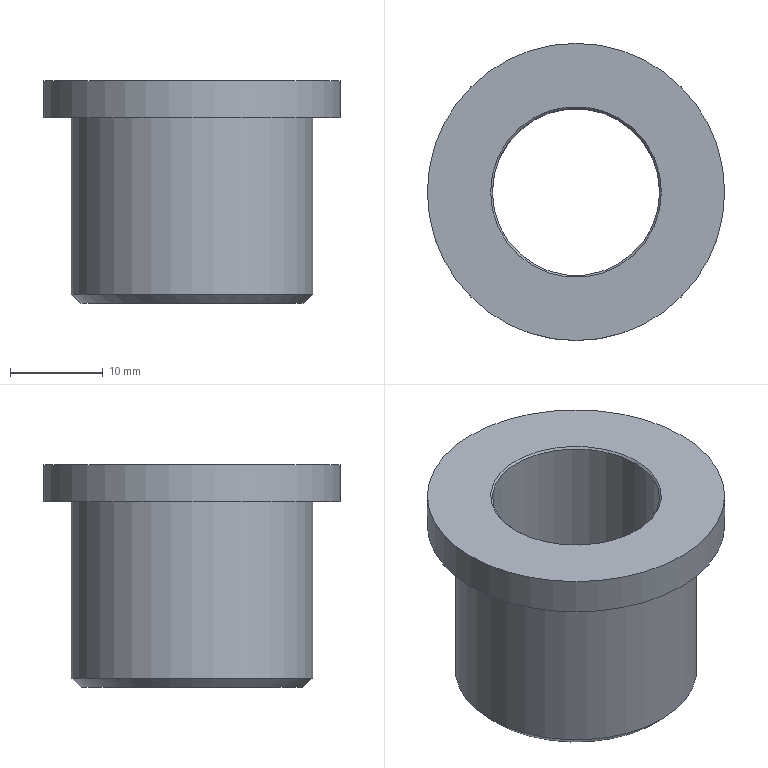Part | NX | features CHAMFER 2, DATUM_CSYS 2, EXTRUDE 2, SKETCH 1 | 1 solid | 9 faces | box 32 x 32 x 24 mm | volume 7686 mm3 | cylinder 3 | plane 3 | cone 3 | commonest cylinder face diameters 18 x1 26 x1 32 x1
STEP:
#1=CARTESIAN_POINT('',(16.,0.,4.));
#2=VERTEX_POINT('',#1);
#3=CARTESIAN_POINT('',(0.,0.,4.));
#4=DIRECTION('',(0.,0.,1.));
#5=DIRECTION('',(1.,0.,0.));
#6=AXIS2_PLACEMENT_3D('',#3,#4,#5);
#7=CIRCLE('',#6,16.);
#8=EDGE_CURVE('',#2,#2,#7,.T.);
#9=ORIENTED_EDGE('',*,*,#8,.F.);
#10=EDGE_LOOP('',(#9));
#11=FACE_BOUND('',#10,.T.);
#12=CARTESIAN_POINT('',(16.,0.,0.));
#13=VERTEX_POINT('',#12);
#14=CARTESIAN_POINT('',(0.,0.,0.));
#15=DIRECTION('',(0.,0.,1.));
#16=DIRECTION('',(1.,0.,0.));
#17=AXIS2_PLACEMENT_3D('',#14,#15,#16);
#18=CIRCLE('',#17,16.);
#19=EDGE_CURVE('',#13,#13,#18,.T.);
#20=ORIENTED_EDGE('',*,*,#19,.T.);
#21=EDGE_LOOP('',(#20));
#22=FACE_BOUND('',#21,.T.);
#23=CARTESIAN_POINT('',(0.,0.,4.));
#24=DIRECTION('',(0.,0.,-1.));
#25=DIRECTION('',(-1.,0.,0.));
#26=AXIS2_PLACEMENT_3D('',#23,#24,#25);
#27=CYLINDRICAL_SURFACE('',#26,16.);
#28=ADVANCED_FACE('',(#11,#22),#27,.T.);
#29=CARTESIAN_POINT('',(-9.,0.,-19.8));
#30=VERTEX_POINT('',#29);
#31=CARTESIAN_POINT('',(0.,0.,-19.8));
#32=DIRECTION('',(0.,0.,-1.));
#33=DIRECTION('',(-1.,0.,0.));
#34=AXIS2_PLACEMENT_3D('',#31,#32,#33);
#35=CIRCLE('',#34,9.);
#36=EDGE_CURVE('',#30,#30,#35,.T.);
#37=ORIENTED_EDGE('',*,*,#36,.T.);
#38=EDGE_LOOP('',(#37));
#39=FACE_BOUND('',#38,.T.);
#40=CARTESIAN_POINT('',(9.,0.,3.8));
#41=VERTEX_POINT('',#40);
#42=CARTESIAN_POINT('',(0.,0.,3.8));
#43=DIRECTION('',(0.,0.,1.));
#44=DIRECTION('',(1.,0.,0.));
#45=AXIS2_PLACEMENT_3D('',#42,#43,#44);
#46=CIRCLE('',#45,9.);
#47=EDGE_CURVE('',#41,#41,#46,.T.);
#48=ORIENTED_EDGE('',*,*,#47,.T.);
#49=EDGE_LOOP('',(#48));
#50=FACE_BOUND('',#49,.T.);
#51=CARTESIAN_POINT('',(0.,0.,4.));
#52=DIRECTION('',(0.,0.,-1.));
#53=DIRECTION('',(-1.,0.,0.));
#54=AXIS2_PLACEMENT_3D('',#51,#52,#53);
#55=CYLINDRICAL_SURFACE('',#54,9.);
#56=ADVANCED_FACE('',(#39,#50),#55,.F.);
#57=CARTESIAN_POINT('',(9.2,0.,4.));
#58=VERTEX_POINT('',#57);
#59=CARTESIAN_POINT('',(0.,0.,4.));
#60=DIRECTION('',(0.,0.,1.));
#61=DIRECTION('',(1.,0.,0.));
#62=AXIS2_PLACEMENT_3D('',#59,#60,#61);
#63=CIRCLE('',#62,9.2);
#64=EDGE_CURVE('',#58,#58,#63,.F.);
#65=ORIENTED_EDGE('',*,*,#64,.T.);
#66=EDGE_LOOP('',(#65));
#67=FACE_BOUND('',#66,.T.);
#68=ORIENTED_EDGE('',*,*,#8,.T.);
#69=EDGE_LOOP('',(#68));
#70=FACE_BOUND('',#69,.T.);
#71=CARTESIAN_POINT('',(0.,0.,4.));
#72=DIRECTION('',(0.,0.,1.));
#73=DIRECTION('',(1.,0.,0.));
#74=AXIS2_PLACEMENT_3D('',#71,#72,#73);
#75=PLANE('',#74);
#76=ADVANCED_FACE('',(#67,#70),#75,.T.);
#77=CARTESIAN_POINT('',(13.,0.,0.));
#78=VERTEX_POINT('',#77);
#79=CARTESIAN_POINT('',(0.,0.,0.));
#80=DIRECTION('',(0.,0.,-1.));
#81=DIRECTION('',(1.,0.,0.));
#82=AXIS2_PLACEMENT_3D('',#79,#80,#81);
#83=CIRCLE('',#82,13.);
#84=EDGE_CURVE('',#78,#78,#83,.T.);
#85=ORIENTED_EDGE('',*,*,#84,.F.);
#86=EDGE_LOOP('',(#85));
#87=FACE_BOUND('',#86,.T.);
#88=ORIENTED_EDGE('',*,*,#19,.F.);
#89=EDGE_LOOP('',(#88));
#90=FACE_BOUND('',#89,.T.);
#91=CARTESIAN_POINT('',(0.,0.,0.));
#92=DIRECTION('',(0.,0.,1.));
#93=DIRECTION('',(1.,0.,0.));
#94=AXIS2_PLACEMENT_3D('',#91,#92,#93);
#95=PLANE('',#94);
#96=ADVANCED_FACE('',(#87,#90),#95,.F.);
#97=CARTESIAN_POINT('',(-13.,0.,-19.));
#98=VERTEX_POINT('',#97);
#99=CARTESIAN_POINT('',(0.,0.,-19.));
#100=DIRECTION('',(0.,0.,-1.));
#101=DIRECTION('',(-1.,0.,0.));
#102=AXIS2_PLACEMENT_3D('',#99,#100,#101);
#103=CIRCLE('',#102,13.);
#104=EDGE_CURVE('',#98,#98,#103,.F.);
#105=ORIENTED_EDGE('',*,*,#104,.T.);
#106=EDGE_LOOP('',(#105));
#107=FACE_BOUND('',#106,.T.);
#108=ORIENTED_EDGE('',*,*,#84,.T.);
#109=EDGE_LOOP('',(#108));
#110=FACE_BOUND('',#109,.T.);
#111=CARTESIAN_POINT('',(0.,0.,-20.));
#112=DIRECTION('',(0.,0.,1.));
#113=DIRECTION('',(1.,0.,0.));
#114=AXIS2_PLACEMENT_3D('',#111,#112,#113);
#115=CYLINDRICAL_SURFACE('',#114,13.);
#116=ADVANCED_FACE('',(#107,#110),#115,.T.);
#117=CARTESIAN_POINT('',(-9.2,0.,-20.));
#118=VERTEX_POINT('',#117);
#119=CARTESIAN_POINT('',(0.,0.,-20.));
#120=DIRECTION('',(0.,0.,-1.));
#121=DIRECTION('',(-1.,0.,0.));
#122=AXIS2_PLACEMENT_3D('',#119,#120,#121);
#123=CIRCLE('',#122,9.2);
#124=EDGE_CURVE('',#118,#118,#123,.F.);
#125=ORIENTED_EDGE('',*,*,#124,.T.);
#126=EDGE_LOOP('',(#125));
#127=FACE_BOUND('',#126,.T.);
#128=CARTESIAN_POINT('',(-12.,0.,-20.));
#129=VERTEX_POINT('',#128);
#130=CARTESIAN_POINT('',(0.,0.,-20.));
#131=DIRECTION('',(0.,0.,-1.));
#132=DIRECTION('',(-1.,0.,0.));
#133=AXIS2_PLACEMENT_3D('',#130,#131,#132);
#134=CIRCLE('',#133,12.);
#135=EDGE_CURVE('',#129,#129,#134,.T.);
#136=ORIENTED_EDGE('',*,*,#135,.T.);
#137=EDGE_LOOP('',(#136));
#138=FACE_BOUND('',#137,.T.);
#139=CARTESIAN_POINT('',(0.,0.,-20.));
#140=DIRECTION('',(0.,0.,-1.));
#141=DIRECTION('',(-1.,0.,0.));
#142=AXIS2_PLACEMENT_3D('',#139,#140,#141);
#143=PLANE('',#142);
#144=ADVANCED_FACE('',(#127,#138),#143,.T.);
#145=ORIENTED_EDGE('',*,*,#104,.F.);
#146=EDGE_LOOP('',(#145));
#147=FACE_BOUND('',#146,.T.);
#148=ORIENTED_EDGE('',*,*,#135,.F.);
#149=EDGE_LOOP('',(#148));
#150=FACE_BOUND('',#149,.T.);
#151=CARTESIAN_POINT('',(0.,0.,-20.));
#152=DIRECTION('',(0.,0.,1.));
#153=DIRECTION('',(1.,0.,0.));
#154=AXIS2_PLACEMENT_3D('',#151,#152,#153);
#155=CONICAL_SURFACE('',#154,12.,0.7854);
#156=ADVANCED_FACE('',(#147,#150),#155,.T.);
#157=ORIENTED_EDGE('',*,*,#36,.F.);
#158=EDGE_LOOP('',(#157));
#159=FACE_BOUND('',#158,.T.);
#160=ORIENTED_EDGE('',*,*,#124,.F.);
#161=EDGE_LOOP('',(#160));
#162=FACE_BOUND('',#161,.T.);
#163=CARTESIAN_POINT('',(0.,0.,-20.));
#164=DIRECTION('',(0.,0.,-1.));
#165=DIRECTION('',(-1.,0.,0.));
#166=AXIS2_PLACEMENT_3D('',#163,#164,#165);
#167=CONICAL_SURFACE('',#166,9.2,0.7854);
#168=ADVANCED_FACE('',(#159,#162),#167,.F.);
#169=ORIENTED_EDGE('',*,*,#64,.F.);
#170=EDGE_LOOP('',(#169));
#171=FACE_BOUND('',#170,.T.);
#172=ORIENTED_EDGE('',*,*,#47,.F.);
#173=EDGE_LOOP('',(#172));
#174=FACE_BOUND('',#173,.T.);
#175=CARTESIAN_POINT('',(0.,0.,3.8));
#176=DIRECTION('',(0.,0.,1.));
#177=DIRECTION('',(1.,0.,0.));
#178=AXIS2_PLACEMENT_3D('',#175,#176,#177);
#179=CONICAL_SURFACE('',#178,9.,0.7854);
#180=ADVANCED_FACE('',(#171,#174),#179,.F.);
#181=CLOSED_SHELL('',(#28,#56,#76,#96,#116,#144,#156,#168,#180));
#182=MANIFOLD_SOLID_BREP('',#181);
#183=(LENGTH_UNIT()NAMED_UNIT(*)SI_UNIT(.MILLI.,.METRE.));
#184=UNCERTAINTY_MEASURE_WITH_UNIT(LENGTH_MEASURE(0.00001),#183,'','');
#185=(NAMED_UNIT(*)PLANE_ANGLE_UNIT()SI_UNIT($,.RADIAN.));
#186=(NAMED_UNIT(*)SI_UNIT($,.STERADIAN.)SOLID_ANGLE_UNIT());
#187=(GEOMETRIC_REPRESENTATION_CONTEXT(3)GLOBAL_UNCERTAINTY_ASSIGNED_CONTEXT((#184))GLOBAL_UNIT_ASSIGNED_CONTEXT((#183,#185,#186))REPRESENTATION_CONTEXT('',''));
#188=ADVANCED_BREP_SHAPE_REPRESENTATION('',(#182),#187);